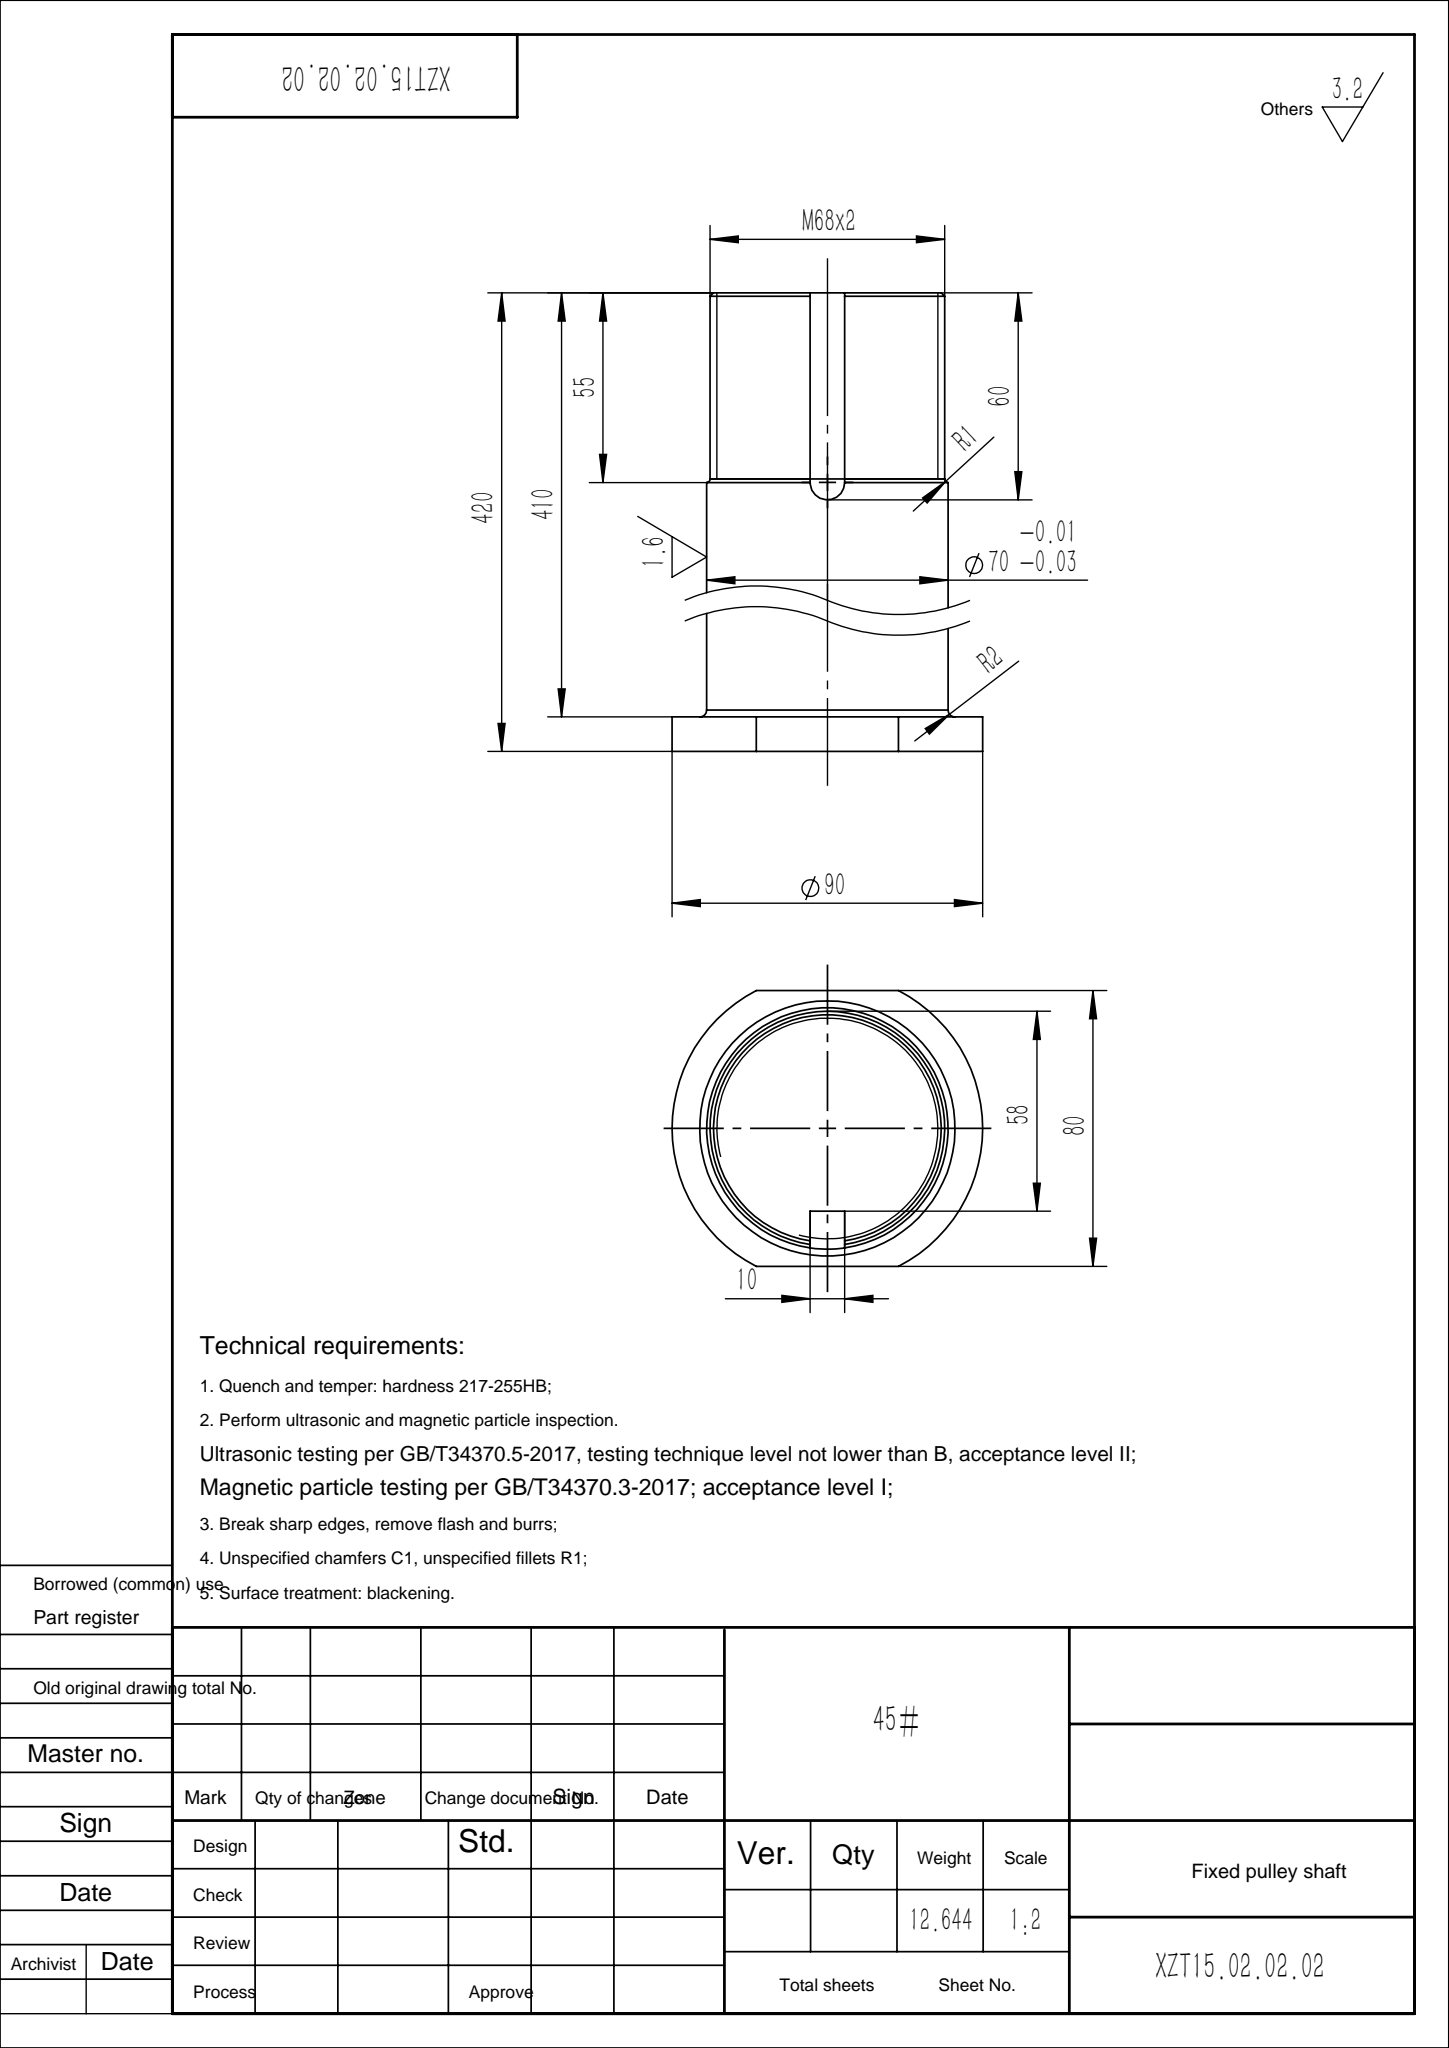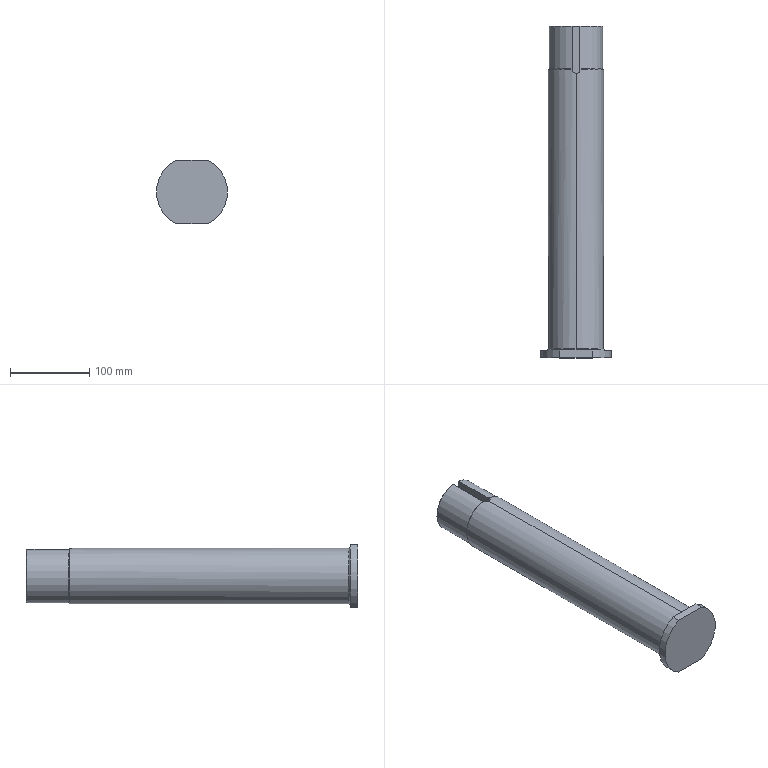Part | SolidWorks | features Fillet 2, ICE 2, Chamfer 1, Revolution 1 | 1 solid | 20 faces | box 90 x 420 x 80 mm | volume 1621053 mm3 | plane 8 | cylinder 6 | torus 4 | cone 2 | commonest cylinder face diameters 70 x2 90 x2 10 x1 68 x1
STEP:
#1=CARTESIAN_POINT('',(0.,10.,37.));
#2=VERTEX_POINT('',#1);
#3=CARTESIAN_POINT('',(0.,10.,-37.));
#4=VERTEX_POINT('',#3);
#5=CARTESIAN_POINT('',(0.,10.,0.));
#6=DIRECTION('',(0.,-1.,0.));
#7=DIRECTION('',(0.,0.,-1.));
#8=AXIS2_PLACEMENT_3D('',#5,#6,#7);
#9=CIRCLE('',#8,37.);
#10=EDGE_CURVE('',#2,#4,#9,.T.);
#11=ORIENTED_EDGE('',*,*,#10,.F.);
#12=CARTESIAN_POINT('',(0.,12.,35.));
#13=VERTEX_POINT('',#12);
#14=CARTESIAN_POINT('',(0.,12.,37.));
#15=DIRECTION('',(1.,0.,0.));
#16=DIRECTION('',(0.,0.,-1.));
#17=AXIS2_PLACEMENT_3D('',#14,#15,#16);
#18=CIRCLE('',#17,2.);
#19=EDGE_CURVE('',#2,#13,#18,.T.);
#20=ORIENTED_EDGE('',*,*,#19,.T.);
#21=CARTESIAN_POINT('',(0.,12.,-35.));
#22=VERTEX_POINT('',#21);
#23=CARTESIAN_POINT('',(0.,12.,0.));
#24=DIRECTION('',(0.,1.,0.));
#25=DIRECTION('',(0.,0.,-1.));
#26=AXIS2_PLACEMENT_3D('',#23,#24,#25);
#27=CIRCLE('',#26,35.);
#28=EDGE_CURVE('',#22,#13,#27,.T.);
#29=ORIENTED_EDGE('',*,*,#28,.F.);
#30=CARTESIAN_POINT('',(0.,12.,-37.));
#31=DIRECTION('',(-1.,0.,0.));
#32=DIRECTION('',(0.,0.,1.));
#33=AXIS2_PLACEMENT_3D('',#30,#31,#32);
#34=CIRCLE('',#33,2.);
#35=EDGE_CURVE('',#4,#22,#34,.T.);
#36=ORIENTED_EDGE('',*,*,#35,.F.);
#37=EDGE_LOOP('',(#11,#20,#29,#36));
#38=FACE_OUTER_BOUND('',#37,.T.);
#39=CARTESIAN_POINT('',(0.,12.,0.));
#40=DIRECTION('',(0.,-1.,0.));
#41=DIRECTION('',(0.,0.,-1.));
#42=AXIS2_PLACEMENT_3D('',#39,#40,#41);
#43=TOROIDAL_SURFACE('',#42,37.,2.);
#44=ADVANCED_FACE('',(#38),#43,.F.);
#45=CARTESIAN_POINT('',(5.,365.,34.641));
#46=VERTEX_POINT('',#45);
#47=CARTESIAN_POINT('',(0.,365.,-35.));
#48=VERTEX_POINT('',#47);
#49=CARTESIAN_POINT('',(0.,365.,0.));
#50=DIRECTION('',(0.,1.,0.));
#51=DIRECTION('',(0.,0.,1.));
#52=AXIS2_PLACEMENT_3D('',#49,#50,#51);
#53=CIRCLE('',#52,35.);
#54=EDGE_CURVE('',#46,#48,#53,.T.);
#55=ORIENTED_EDGE('',*,*,#54,.T.);
#56=CARTESIAN_POINT('',(0.,366.,-34.));
#57=VERTEX_POINT('',#56);
#58=CARTESIAN_POINT('',(0.,366.,-35.));
#59=DIRECTION('',(-1.,0.,0.));
#60=DIRECTION('',(0.,0.,1.));
#61=AXIS2_PLACEMENT_3D('',#58,#59,#60);
#62=CIRCLE('',#61,1.);
#63=EDGE_CURVE('',#48,#57,#62,.T.);
#64=ORIENTED_EDGE('',*,*,#63,.T.);
#65=CARTESIAN_POINT('',(5.,366.,33.63));
#66=VERTEX_POINT('',#65);
#67=CARTESIAN_POINT('',(0.,366.,0.));
#68=DIRECTION('',(0.,1.,0.));
#69=DIRECTION('',(0.,0.,-1.));
#70=AXIS2_PLACEMENT_3D('',#67,#68,#69);
#71=CIRCLE('',#70,34.);
#72=EDGE_CURVE('',#66,#57,#71,.T.);
#73=ORIENTED_EDGE('',*,*,#72,.F.);
#74=CARTESIAN_POINT('',(5.,365.,34.641));
#75=CARTESIAN_POINT('',(5.,365.,34.508));
#76=CARTESIAN_POINT('',(5.,365.026,34.378));
#77=CARTESIAN_POINT('',(5.,365.125,34.134));
#78=CARTESIAN_POINT('',(5.,365.199,34.022));
#79=CARTESIAN_POINT('',(5.,365.475,33.742));
#80=CARTESIAN_POINT('',(5.,365.734,33.63));
#81=CARTESIAN_POINT('',(5.,366.,33.63));
#82=B_SPLINE_CURVE_WITH_KNOTS('',3,(#74,#75,#76,#77,#78,#79,#80,#81),.UNSPECIFIED.,.F.,.F.,(4,2,2,4),(0.,0.0003926,0.0007852,0.00157),.UNSPECIFIED.);
#83=EDGE_CURVE('',#46,#66,#82,.T.);
#84=ORIENTED_EDGE('',*,*,#83,.F.);
#85=EDGE_LOOP('',(#55,#64,#73,#84));
#86=FACE_OUTER_BOUND('',#85,.T.);
#87=CARTESIAN_POINT('',(0.,366.,0.));
#88=DIRECTION('',(0.,-1.,0.));
#89=DIRECTION('',(0.,0.,-1.));
#90=AXIS2_PLACEMENT_3D('',#87,#88,#89);
#91=TOROIDAL_SURFACE('',#90,35.,1.);
#92=ADVANCED_FACE('',(#86),#91,.F.);
#93=CARTESIAN_POINT('',(0.,420.,-33.));
#94=VERTEX_POINT('',#93);
#95=CARTESIAN_POINT('',(-5.,420.,32.619));
#96=VERTEX_POINT('',#95);
#97=CARTESIAN_POINT('',(0.,420.,0.));
#98=DIRECTION('',(0.,1.,0.));
#99=DIRECTION('',(0.,0.,-1.));
#100=AXIS2_PLACEMENT_3D('',#97,#98,#99);
#101=CIRCLE('',#100,33.);
#102=EDGE_CURVE('',#94,#96,#101,.T.);
#103=ORIENTED_EDGE('',*,*,#102,.F.);
#104=CARTESIAN_POINT('',(0.,419.,-34.));
#105=VERTEX_POINT('',#104);
#106=CARTESIAN_POINT('',(0.,420.,-33.));
#107=DIRECTION('',(0.,-0.7071,-0.7071));
#108=VECTOR('',#107,1000.);
#109=LINE('',#106,#108);
#110=EDGE_CURVE('',#94,#105,#109,.T.);
#111=ORIENTED_EDGE('',*,*,#110,.T.);
#112=CARTESIAN_POINT('',(-5.,419.,33.63));
#113=VERTEX_POINT('',#112);
#114=CARTESIAN_POINT('',(0.,419.,0.));
#115=DIRECTION('',(0.,-1.,0.));
#116=DIRECTION('',(0.,0.,-1.));
#117=AXIS2_PLACEMENT_3D('',#114,#115,#116);
#118=CIRCLE('',#117,34.);
#119=EDGE_CURVE('',#113,#105,#118,.T.);
#120=ORIENTED_EDGE('',*,*,#119,.F.);
#121=CARTESIAN_POINT('',(-5.,420.,32.619));
#122=CARTESIAN_POINT('',(-5.,419.667,32.956));
#123=CARTESIAN_POINT('',(-5.,419.333,33.293));
#124=CARTESIAN_POINT('',(-5.,419.,33.63));
#125=B_SPLINE_CURVE_WITH_KNOTS('',3,(#121,#122,#123,#124),.UNSPECIFIED.,.F.,.F.,(4,4),(0.,0.001422),.UNSPECIFIED.);
#126=EDGE_CURVE('',#96,#113,#125,.T.);
#127=ORIENTED_EDGE('',*,*,#126,.F.);
#128=EDGE_LOOP('',(#103,#111,#120,#127));
#129=FACE_OUTER_BOUND('',#128,.T.);
#130=CARTESIAN_POINT('',(0.,420.,0.));
#131=DIRECTION('',(0.,-1.,0.));
#132=DIRECTION('',(0.,0.,-1.));
#133=AXIS2_PLACEMENT_3D('',#130,#131,#132);
#134=CONICAL_SURFACE('',#133,33.,0.7854);
#135=ADVANCED_FACE('',(#129),#134,.T.);
#136=CARTESIAN_POINT('',(0.,12.,0.));
#137=DIRECTION('',(0.,1.,0.));
#138=DIRECTION('',(0.,0.,-1.));
#139=AXIS2_PLACEMENT_3D('',#136,#137,#138);
#140=CIRCLE('',#139,35.);
#141=EDGE_CURVE('',#13,#22,#140,.T.);
#142=ORIENTED_EDGE('',*,*,#141,.T.);
#143=CARTESIAN_POINT('',(0.,0.,-35.));
#144=DIRECTION('',(0.,1.,0.));
#145=VECTOR('',#144,1000.);
#146=LINE('',#143,#145);
#147=EDGE_CURVE('',#22,#48,#146,.T.);
#148=ORIENTED_EDGE('',*,*,#147,.T.);
#149=ORIENTED_EDGE('',*,*,#54,.F.);
#150=CARTESIAN_POINT('',(0.,360.,35.));
#151=VERTEX_POINT('',#150);
#152=CARTESIAN_POINT('',(5.,365.,34.641));
#153=CARTESIAN_POINT('',(5.,364.669,34.641));
#154=CARTESIAN_POINT('',(4.967,364.344,34.646));
#155=CARTESIAN_POINT('',(4.872,363.864,34.659));
#156=CARTESIAN_POINT('',(4.832,363.705,34.665));
#157=CARTESIAN_POINT('',(4.737,363.391,34.678));
#158=CARTESIAN_POINT('',(4.681,363.235,34.686));
#159=CARTESIAN_POINT('',(4.492,362.781,34.711));
#160=CARTESIAN_POINT('',(4.339,362.494,34.731));
#161=CARTESIAN_POINT('',(3.976,361.95,34.774));
#162=CARTESIAN_POINT('',(3.765,361.693,34.798));
#163=CARTESIAN_POINT('',(3.304,361.233,34.845));
#164=CARTESIAN_POINT('',(3.052,361.026,34.868));
#165=CARTESIAN_POINT('',(2.505,360.66,34.911));
#166=CARTESIAN_POINT('',(2.215,360.505,34.931));
#167=CARTESIAN_POINT('',(1.613,360.256,34.964));
#168=CARTESIAN_POINT('',(1.297,360.16,34.977));
#169=CARTESIAN_POINT('',(0.6515,360.032,34.995));
#170=CARTESIAN_POINT('',(0.3267,360.,35.));
#171=CARTESIAN_POINT('',(0.,360.,35.));
#172=B_SPLINE_CURVE_WITH_KNOTS('',3,(#152,#153,#154,#155,#156,#157,#158,#159,#160,#161,#162,#163,#164,#165,#166,#167,#168,#169,#170,#171),.UNSPECIFIED.,.F.,.F.,(4,2,2,2,2,2,2,2,2,4),(0.,0.0009785,0.001468,0.001957,0.002935,0.003914,0.004892,0.005871,0.006849,0.007828),.UNSPECIFIED.);
#173=EDGE_CURVE('',#46,#151,#172,.T.);
#174=ORIENTED_EDGE('',*,*,#173,.T.);
#175=CARTESIAN_POINT('',(0.,0.,35.));
#176=DIRECTION('',(0.,1.,0.));
#177=VECTOR('',#176,1000.);
#178=LINE('',#175,#177);
#179=EDGE_CURVE('',#13,#151,#178,.T.);
#180=ORIENTED_EDGE('',*,*,#179,.F.);
#181=EDGE_LOOP('',(#142,#148,#149,#174,#180));
#182=FACE_OUTER_BOUND('',#181,.T.);
#183=CARTESIAN_POINT('',(0.,0.,0.));
#184=DIRECTION('',(0.,1.,0.));
#185=DIRECTION('',(0.,0.,1.));
#186=AXIS2_PLACEMENT_3D('',#183,#184,#185);
#187=CYLINDRICAL_SURFACE('',#186,35.);
#188=ADVANCED_FACE('',(#182),#187,.T.);
#189=ORIENTED_EDGE('',*,*,#147,.F.);
#190=ORIENTED_EDGE('',*,*,#28,.T.);
#191=ORIENTED_EDGE('',*,*,#179,.T.);
#192=CARTESIAN_POINT('',(-5.,365.,34.641));
#193=VERTEX_POINT('',#192);
#194=CARTESIAN_POINT('',(0.,360.,35.));
#195=CARTESIAN_POINT('',(-0.3264,360.,35.));
#196=CARTESIAN_POINT('',(-0.6579,360.033,34.995));
#197=CARTESIAN_POINT('',(-1.299,360.161,34.977));
#198=CARTESIAN_POINT('',(-1.611,360.255,34.964));
#199=CARTESIAN_POINT('',(-2.065,360.443,34.939));
#200=CARTESIAN_POINT('',(-2.215,360.514,34.93));
#201=CARTESIAN_POINT('',(-2.504,360.669,34.911));
#202=CARTESIAN_POINT('',(-2.643,360.753,34.9));
#203=CARTESIAN_POINT('',(-3.049,361.024,34.868));
#204=CARTESIAN_POINT('',(-3.302,361.231,34.845));
#205=CARTESIAN_POINT('',(-3.768,361.696,34.797));
#206=CARTESIAN_POINT('',(-3.974,361.948,34.774));
#207=CARTESIAN_POINT('',(-4.336,362.489,34.731));
#208=CARTESIAN_POINT('',(-4.493,362.781,34.711));
#209=CARTESIAN_POINT('',(-4.744,363.386,34.677));
#210=CARTESIAN_POINT('',(-4.838,363.697,34.664));
#211=CARTESIAN_POINT('',(-4.967,364.338,34.646));
#212=CARTESIAN_POINT('',(-5.,364.669,34.641));
#213=CARTESIAN_POINT('',(-5.,365.,34.641));
#214=B_SPLINE_CURVE_WITH_KNOTS('',3,(#194,#195,#196,#197,#198,#199,#200,#201,#202,#203,#204,#205,#206,#207,#208,#209,#210,#211,#212,#213),.UNSPECIFIED.,.F.,.F.,(4,2,2,2,2,2,2,2,2,4),(0.007828,0.008806,0.009783,0.01027,0.01076,0.01174,0.01272,0.01369,0.01467,0.01565),.UNSPECIFIED.);
#215=EDGE_CURVE('',#151,#193,#214,.T.);
#216=ORIENTED_EDGE('',*,*,#215,.T.);
#217=CARTESIAN_POINT('',(0.,365.,0.));
#218=DIRECTION('',(0.,1.,0.));
#219=DIRECTION('',(0.,0.,1.));
#220=AXIS2_PLACEMENT_3D('',#217,#218,#219);
#221=CIRCLE('',#220,35.);
#222=EDGE_CURVE('',#48,#193,#221,.T.);
#223=ORIENTED_EDGE('',*,*,#222,.F.);
#224=EDGE_LOOP('',(#189,#190,#191,#216,#223));
#225=FACE_OUTER_BOUND('',#224,.T.);
#226=CARTESIAN_POINT('',(0.,0.,0.));
#227=DIRECTION('',(0.,1.,0.));
#228=DIRECTION('',(0.,0.,1.));
#229=AXIS2_PLACEMENT_3D('',#226,#227,#228);
#230=CYLINDRICAL_SURFACE('',#229,35.);
#231=ADVANCED_FACE('',(#225),#230,.T.);
#232=CARTESIAN_POINT('',(5.,419.,33.63));
#233=VERTEX_POINT('',#232);
#234=CARTESIAN_POINT('',(5.,0.,33.63));
#235=DIRECTION('',(0.,-1.,0.));
#236=VECTOR('',#235,1000.);
#237=LINE('',#234,#236);
#238=EDGE_CURVE('',#233,#66,#237,.T.);
#239=ORIENTED_EDGE('',*,*,#238,.T.);
#240=ORIENTED_EDGE('',*,*,#72,.T.);
#241=CARTESIAN_POINT('',(-5.,366.,33.63));
#242=VERTEX_POINT('',#241);
#243=CARTESIAN_POINT('',(0.,366.,0.));
#244=DIRECTION('',(0.,1.,0.));
#245=DIRECTION('',(0.,0.,-1.));
#246=AXIS2_PLACEMENT_3D('',#243,#244,#245);
#247=CIRCLE('',#246,34.);
#248=EDGE_CURVE('',#57,#242,#247,.T.);
#249=ORIENTED_EDGE('',*,*,#248,.T.);
#250=CARTESIAN_POINT('',(-5.,0.,33.63));
#251=DIRECTION('',(0.,1.,0.));
#252=VECTOR('',#251,1000.);
#253=LINE('',#250,#252);
#254=EDGE_CURVE('',#242,#113,#253,.T.);
#255=ORIENTED_EDGE('',*,*,#254,.T.);
#256=ORIENTED_EDGE('',*,*,#119,.T.);
#257=CARTESIAN_POINT('',(0.,419.,0.));
#258=DIRECTION('',(0.,-1.,0.));
#259=DIRECTION('',(0.,0.,-1.));
#260=AXIS2_PLACEMENT_3D('',#257,#258,#259);
#261=CIRCLE('',#260,34.);
#262=EDGE_CURVE('',#105,#233,#261,.T.);
#263=ORIENTED_EDGE('',*,*,#262,.T.);
#264=EDGE_LOOP('',(#239,#240,#249,#255,#256,#263));
#265=FACE_OUTER_BOUND('',#264,.T.);
#266=CARTESIAN_POINT('',(0.,0.,0.));
#267=DIRECTION('',(0.,1.,0.));
#268=DIRECTION('',(0.,0.,1.));
#269=AXIS2_PLACEMENT_3D('',#266,#267,#268);
#270=CYLINDRICAL_SURFACE('',#269,34.);
#271=ADVANCED_FACE('',(#265),#270,.T.);
#272=CARTESIAN_POINT('',(5.,420.,24.));
#273=VERTEX_POINT('',#272);
#274=CARTESIAN_POINT('',(5.,420.,32.619));
#275=VERTEX_POINT('',#274);
#276=CARTESIAN_POINT('',(5.,420.,40.001));
#277=DIRECTION('',(0.,0.,1.));
#278=VECTOR('',#277,1000.);
#279=LINE('',#276,#278);
#280=EDGE_CURVE('',#273,#275,#279,.T.);
#281=ORIENTED_EDGE('',*,*,#280,.T.);
#282=CARTESIAN_POINT('',(0.,420.,0.));
#283=DIRECTION('',(0.,1.,0.));
#284=DIRECTION('',(0.,0.,-1.));
#285=AXIS2_PLACEMENT_3D('',#282,#283,#284);
#286=CIRCLE('',#285,33.);
#287=EDGE_CURVE('',#275,#94,#286,.T.);
#288=ORIENTED_EDGE('',*,*,#287,.T.);
#289=ORIENTED_EDGE('',*,*,#102,.T.);
#290=CARTESIAN_POINT('',(-5.,420.,24.));
#291=VERTEX_POINT('',#290);
#292=CARTESIAN_POINT('',(-5.,420.,40.001));
#293=DIRECTION('',(0.,0.,-1.));
#294=VECTOR('',#293,1000.);
#295=LINE('',#292,#294);
#296=EDGE_CURVE('',#96,#291,#295,.T.);
#297=ORIENTED_EDGE('',*,*,#296,.T.);
#298=CARTESIAN_POINT('',(0.,420.,24.));
#299=DIRECTION('',(1.,0.,0.));
#300=VECTOR('',#299,1000.);
#301=LINE('',#298,#300);
#302=EDGE_CURVE('',#291,#273,#301,.T.);
#303=ORIENTED_EDGE('',*,*,#302,.T.);
#304=EDGE_LOOP('',(#281,#288,#289,#297,#303));
#305=FACE_OUTER_BOUND('',#304,.T.);
#306=CARTESIAN_POINT('',(34.,420.,0.));
#307=DIRECTION('',(0.,-1.,0.));
#308=DIRECTION('',(0.,0.,-1.));
#309=AXIS2_PLACEMENT_3D('',#306,#307,#308);
#310=PLANE('',#309);
#311=ADVANCED_FACE('',(#305),#310,.F.);
#312=CARTESIAN_POINT('',(-20.616,0.,-40.));
#313=VERTEX_POINT('',#312);
#314=CARTESIAN_POINT('',(-20.616,0.,40.));
#315=VERTEX_POINT('',#314);
#316=CARTESIAN_POINT('',(0.,0.,0.));
#317=DIRECTION('',(0.,1.,0.));
#318=DIRECTION('',(0.,0.,1.));
#319=AXIS2_PLACEMENT_3D('',#316,#317,#318);
#320=CIRCLE('',#319,45.);
#321=EDGE_CURVE('',#313,#315,#320,.T.);
#322=ORIENTED_EDGE('',*,*,#321,.T.);
#323=CARTESIAN_POINT('',(-20.616,10.,40.));
#324=VERTEX_POINT('',#323);
#325=CARTESIAN_POINT('',(-20.616,0.,40.));
#326=DIRECTION('',(0.,1.,0.));
#327=VECTOR('',#326,1000.);
#328=LINE('',#325,#327);
#329=EDGE_CURVE('',#315,#324,#328,.T.);
#330=ORIENTED_EDGE('',*,*,#329,.T.);
#331=CARTESIAN_POINT('',(-20.616,10.,-40.));
#332=VERTEX_POINT('',#331);
#333=CARTESIAN_POINT('',(0.,10.,0.));
#334=DIRECTION('',(0.,1.,0.));
#335=DIRECTION('',(0.,0.,1.));
#336=AXIS2_PLACEMENT_3D('',#333,#334,#335);
#337=CIRCLE('',#336,45.);
#338=EDGE_CURVE('',#332,#324,#337,.T.);
#339=ORIENTED_EDGE('',*,*,#338,.F.);
#340=CARTESIAN_POINT('',(-20.616,0.,-40.));
#341=DIRECTION('',(0.,-1.,0.));
#342=VECTOR('',#341,1000.);
#343=LINE('',#340,#342);
#344=EDGE_CURVE('',#332,#313,#343,.T.);
#345=ORIENTED_EDGE('',*,*,#344,.T.);
#346=EDGE_LOOP('',(#322,#330,#339,#345));
#347=FACE_OUTER_BOUND('',#346,.T.);
#348=CARTESIAN_POINT('',(0.,0.,0.));
#349=DIRECTION('',(0.,1.,0.));
#350=DIRECTION('',(0.,0.,1.));
#351=AXIS2_PLACEMENT_3D('',#348,#349,#350);
#352=CYLINDRICAL_SURFACE('',#351,45.);
#353=ADVANCED_FACE('',(#347),#352,.T.);
#354=CARTESIAN_POINT('',(20.616,0.,40.));
#355=VERTEX_POINT('',#354);
#356=CARTESIAN_POINT('',(20.616,0.,-40.));
#357=VERTEX_POINT('',#356);
#358=CARTESIAN_POINT('',(0.,0.,0.));
#359=DIRECTION('',(0.,1.,0.));
#360=DIRECTION('',(0.,0.,1.));
#361=AXIS2_PLACEMENT_3D('',#358,#359,#360);
#362=CIRCLE('',#361,45.);
#363=EDGE_CURVE('',#355,#357,#362,.T.);
#364=ORIENTED_EDGE('',*,*,#363,.F.);
#365=CARTESIAN_POINT('',(65.,0.,40.));
#366=DIRECTION('',(1.,0.,0.));
#367=VECTOR('',#366,1000.);
#368=LINE('',#365,#367);
#369=EDGE_CURVE('',#315,#355,#368,.T.);
#370=ORIENTED_EDGE('',*,*,#369,.F.);
#371=ORIENTED_EDGE('',*,*,#321,.F.);
#372=CARTESIAN_POINT('',(65.,0.,-40.));
#373=DIRECTION('',(-1.,0.,0.));
#374=VECTOR('',#373,1000.);
#375=LINE('',#372,#374);
#376=EDGE_CURVE('',#357,#313,#375,.T.);
#377=ORIENTED_EDGE('',*,*,#376,.F.);
#378=EDGE_LOOP('',(#364,#370,#371,#377));
#379=FACE_OUTER_BOUND('',#378,.T.);
#380=CARTESIAN_POINT('',(0.,0.,0.));
#381=DIRECTION('',(0.,1.,0.));
#382=DIRECTION('',(0.,0.,1.));
#383=AXIS2_PLACEMENT_3D('',#380,#381,#382);
#384=PLANE('',#383);
#385=ADVANCED_FACE('',(#379),#384,.F.);
#386=CARTESIAN_POINT('',(20.616,10.,40.));
#387=VERTEX_POINT('',#386);
#388=CARTESIAN_POINT('',(20.616,10.,-40.));
#389=VERTEX_POINT('',#388);
#390=CARTESIAN_POINT('',(0.,10.,0.));
#391=DIRECTION('',(0.,1.,0.));
#392=DIRECTION('',(0.,0.,1.));
#393=AXIS2_PLACEMENT_3D('',#390,#391,#392);
#394=CIRCLE('',#393,45.);
#395=EDGE_CURVE('',#387,#389,#394,.T.);
#396=ORIENTED_EDGE('',*,*,#395,.F.);
#397=CARTESIAN_POINT('',(20.616,0.,40.));
#398=DIRECTION('',(0.,-1.,0.));
#399=VECTOR('',#398,1000.);
#400=LINE('',#397,#399);
#401=EDGE_CURVE('',#387,#355,#400,.T.);
#402=ORIENTED_EDGE('',*,*,#401,.T.);
#403=ORIENTED_EDGE('',*,*,#363,.T.);
#404=CARTESIAN_POINT('',(20.616,0.,-40.));
#405=DIRECTION('',(0.,1.,0.));
#406=VECTOR('',#405,1000.);
#407=LINE('',#404,#406);
#408=EDGE_CURVE('',#357,#389,#407,.T.);
#409=ORIENTED_EDGE('',*,*,#408,.T.);
#410=EDGE_LOOP('',(#396,#402,#403,#409));
#411=FACE_OUTER_BOUND('',#410,.T.);
#412=CARTESIAN_POINT('',(0.,0.,0.));
#413=DIRECTION('',(0.,1.,0.));
#414=DIRECTION('',(0.,0.,1.));
#415=AXIS2_PLACEMENT_3D('',#412,#413,#414);
#416=CYLINDRICAL_SURFACE('',#415,45.);
#417=ADVANCED_FACE('',(#411),#416,.T.);
#418=CARTESIAN_POINT('',(0.,10.,0.));
#419=DIRECTION('',(0.,-1.,0.));
#420=DIRECTION('',(0.,0.,-1.));
#421=AXIS2_PLACEMENT_3D('',#418,#419,#420);
#422=CIRCLE('',#421,37.);
#423=EDGE_CURVE('',#4,#2,#422,.T.);
#424=ORIENTED_EDGE('',*,*,#423,.T.);
#425=ORIENTED_EDGE('',*,*,#10,.T.);
#426=EDGE_LOOP('',(#424,#425));
#427=FACE_BOUND('',#426,.T.);
#428=ORIENTED_EDGE('',*,*,#338,.T.);
#429=CARTESIAN_POINT('',(45.,10.,40.));
#430=DIRECTION('',(1.,0.,0.));
#431=VECTOR('',#430,1000.);
#432=LINE('',#429,#431);
#433=EDGE_CURVE('',#324,#387,#432,.T.);
#434=ORIENTED_EDGE('',*,*,#433,.T.);
#435=ORIENTED_EDGE('',*,*,#395,.T.);
#436=CARTESIAN_POINT('',(45.,10.,-40.));
#437=DIRECTION('',(-1.,0.,0.));
#438=VECTOR('',#437,1000.);
#439=LINE('',#436,#438);
#440=EDGE_CURVE('',#389,#332,#439,.T.);
#441=ORIENTED_EDGE('',*,*,#440,.T.);
#442=EDGE_LOOP('',(#428,#434,#435,#441));
#443=FACE_OUTER_BOUND('',#442,.T.);
#444=CARTESIAN_POINT('',(45.,10.,0.));
#445=DIRECTION('',(0.,-1.,0.));
#446=DIRECTION('',(0.,0.,-1.));
#447=AXIS2_PLACEMENT_3D('',#444,#445,#446);
#448=PLANE('',#447);
#449=ADVANCED_FACE('',(#427,#443),#448,.F.);
#450=ORIENTED_EDGE('',*,*,#376,.T.);
#451=ORIENTED_EDGE('',*,*,#344,.F.);
#452=ORIENTED_EDGE('',*,*,#440,.F.);
#453=ORIENTED_EDGE('',*,*,#408,.F.);
#454=EDGE_LOOP('',(#450,#451,#452,#453));
#455=FACE_OUTER_BOUND('',#454,.T.);
#456=CARTESIAN_POINT('',(65.,10.,-40.));
#457=DIRECTION('',(0.,0.,1.));
#458=DIRECTION('',(1.,0.,0.));
#459=AXIS2_PLACEMENT_3D('',#456,#457,#458);
#460=PLANE('',#459);
#461=ADVANCED_FACE('',(#455),#460,.F.);
#462=ORIENTED_EDGE('',*,*,#369,.T.);
#463=ORIENTED_EDGE('',*,*,#401,.F.);
#464=ORIENTED_EDGE('',*,*,#433,.F.);
#465=ORIENTED_EDGE('',*,*,#329,.F.);
#466=EDGE_LOOP('',(#462,#463,#464,#465));
#467=FACE_OUTER_BOUND('',#466,.T.);
#468=CARTESIAN_POINT('',(65.,10.,40.));
#469=DIRECTION('',(0.,0.,-1.));
#470=DIRECTION('',(-1.,0.,0.));
#471=AXIS2_PLACEMENT_3D('',#468,#469,#470);
#472=PLANE('',#471);
#473=ADVANCED_FACE('',(#467),#472,.F.);
#474=ORIENTED_EDGE('',*,*,#296,.F.);
#475=ORIENTED_EDGE('',*,*,#126,.T.);
#476=ORIENTED_EDGE('',*,*,#254,.F.);
#477=CARTESIAN_POINT('',(-5.,366.,33.63));
#478=CARTESIAN_POINT('',(-5.,365.867,33.63));
#479=CARTESIAN_POINT('',(-5.,365.737,33.657));
#480=CARTESIAN_POINT('',(-5.,365.494,33.759));
#481=CARTESIAN_POINT('',(-5.,365.383,33.835));
#482=CARTESIAN_POINT('',(-5.,365.199,34.021));
#483=CARTESIAN_POINT('',(-5.,365.125,34.134));
#484=CARTESIAN_POINT('',(-5.,365.026,34.376));
#485=CARTESIAN_POINT('',(-5.,365.,34.508));
#486=CARTESIAN_POINT('',(-5.,365.,34.641));
#487=B_SPLINE_CURVE_WITH_KNOTS('',3,(#477,#478,#479,#480,#481,#482,#483,#484,#485,#486),.UNSPECIFIED.,.F.,.F.,(4,2,2,2,4),(0.,0.0003926,0.0007852,0.001178,0.00157),.UNSPECIFIED.);
#488=EDGE_CURVE('',#242,#193,#487,.T.);
#489=ORIENTED_EDGE('',*,*,#488,.T.);
#490=CARTESIAN_POINT('',(-5.,365.,24.));
#491=VERTEX_POINT('',#490);
#492=CARTESIAN_POINT('',(-5.,365.,40.001));
#493=DIRECTION('',(0.,0.,-1.));
#494=VECTOR('',#493,1000.);
#495=LINE('',#492,#494);
#496=EDGE_CURVE('',#193,#491,#495,.T.);
#497=ORIENTED_EDGE('',*,*,#496,.T.);
#498=CARTESIAN_POINT('',(-5.,420.,24.));
#499=DIRECTION('',(0.,-1.,0.));
#500=VECTOR('',#499,1000.);
#501=LINE('',#498,#500);
#502=EDGE_CURVE('',#291,#491,#501,.T.);
#503=ORIENTED_EDGE('',*,*,#502,.F.);
#504=EDGE_LOOP('',(#474,#475,#476,#489,#497,#503));
#505=FACE_OUTER_BOUND('',#504,.T.);
#506=CARTESIAN_POINT('',(-5.,420.,40.001));
#507=DIRECTION('',(1.,0.,0.));
#508=DIRECTION('',(0.,1.,0.));
#509=AXIS2_PLACEMENT_3D('',#506,#507,#508);
#510=PLANE('',#509);
#511=ADVANCED_FACE('',(#505),#510,.T.);
#512=ORIENTED_EDGE('',*,*,#173,.F.);
#513=CARTESIAN_POINT('',(5.,365.,24.));
#514=VERTEX_POINT('',#513);
#515=CARTESIAN_POINT('',(5.,365.,40.001));
#516=DIRECTION('',(0.,0.,-1.));
#517=VECTOR('',#516,1000.);
#518=LINE('',#515,#517);
#519=EDGE_CURVE('',#46,#514,#518,.T.);
#520=ORIENTED_EDGE('',*,*,#519,.T.);
#521=CARTESIAN_POINT('',(0.,365.,24.));
#522=DIRECTION('',(0.,0.,1.));
#523=DIRECTION('',(1.,0.,0.));
#524=AXIS2_PLACEMENT_3D('',#521,#522,#523);
#525=CIRCLE('',#524,5.);
#526=EDGE_CURVE('',#491,#514,#525,.T.);
#527=ORIENTED_EDGE('',*,*,#526,.F.);
#528=ORIENTED_EDGE('',*,*,#496,.F.);
#529=ORIENTED_EDGE('',*,*,#215,.F.);
#530=EDGE_LOOP('',(#512,#520,#527,#528,#529));
#531=FACE_OUTER_BOUND('',#530,.T.);
#532=CARTESIAN_POINT('',(0.,365.,40.001));
#533=DIRECTION('',(0.,0.,-1.));
#534=DIRECTION('',(-1.,0.,0.));
#535=AXIS2_PLACEMENT_3D('',#532,#533,#534);
#536=CYLINDRICAL_SURFACE('',#535,5.);
#537=ADVANCED_FACE('',(#531),#536,.F.);
#538=ORIENTED_EDGE('',*,*,#238,.F.);
#539=CARTESIAN_POINT('',(5.,419.,33.63));
#540=CARTESIAN_POINT('',(5.,419.333,33.293));
#541=CARTESIAN_POINT('',(5.,419.667,32.956));
#542=CARTESIAN_POINT('',(5.,420.,32.619));
#543=B_SPLINE_CURVE_WITH_KNOTS('',3,(#539,#540,#541,#542),.UNSPECIFIED.,.F.,.F.,(4,4),(0.,0.001422),.UNSPECIFIED.);
#544=EDGE_CURVE('',#233,#275,#543,.T.);
#545=ORIENTED_EDGE('',*,*,#544,.T.);
#546=ORIENTED_EDGE('',*,*,#280,.F.);
#547=CARTESIAN_POINT('',(5.,420.,24.));
#548=DIRECTION('',(0.,1.,0.));
#549=VECTOR('',#548,1000.);
#550=LINE('',#547,#549);
#551=EDGE_CURVE('',#514,#273,#550,.T.);
#552=ORIENTED_EDGE('',*,*,#551,.F.);
#553=ORIENTED_EDGE('',*,*,#519,.F.);
#554=ORIENTED_EDGE('',*,*,#83,.T.);
#555=EDGE_LOOP('',(#538,#545,#546,#552,#553,#554));
#556=FACE_OUTER_BOUND('',#555,.T.);
#557=CARTESIAN_POINT('',(5.,420.,40.001));
#558=DIRECTION('',(-1.,0.,0.));
#559=DIRECTION('',(0.,-1.,0.));
#560=AXIS2_PLACEMENT_3D('',#557,#558,#559);
#561=PLANE('',#560);
#562=ADVANCED_FACE('',(#556),#561,.T.);
#563=ORIENTED_EDGE('',*,*,#502,.T.);
#564=ORIENTED_EDGE('',*,*,#526,.T.);
#565=ORIENTED_EDGE('',*,*,#551,.T.);
#566=ORIENTED_EDGE('',*,*,#302,.F.);
#567=EDGE_LOOP('',(#563,#564,#565,#566));
#568=FACE_OUTER_BOUND('',#567,.T.);
#569=CARTESIAN_POINT('',(0.,420.,24.));
#570=DIRECTION('',(0.,0.,1.));
#571=DIRECTION('',(1.,0.,0.));
#572=AXIS2_PLACEMENT_3D('',#569,#570,#571);
#573=PLANE('',#572);
#574=ADVANCED_FACE('',(#568),#573,.T.);
#575=ORIENTED_EDGE('',*,*,#110,.F.);
#576=ORIENTED_EDGE('',*,*,#287,.F.);
#577=ORIENTED_EDGE('',*,*,#544,.F.);
#578=ORIENTED_EDGE('',*,*,#262,.F.);
#579=EDGE_LOOP('',(#575,#576,#577,#578));
#580=FACE_OUTER_BOUND('',#579,.T.);
#581=CARTESIAN_POINT('',(0.,420.,0.));
#582=DIRECTION('',(0.,-1.,0.));
#583=DIRECTION('',(0.,0.,-1.));
#584=AXIS2_PLACEMENT_3D('',#581,#582,#583);
#585=CONICAL_SURFACE('',#584,33.,0.7854);
#586=ADVANCED_FACE('',(#580),#585,.T.);
#587=ORIENTED_EDGE('',*,*,#63,.F.);
#588=ORIENTED_EDGE('',*,*,#222,.T.);
#589=ORIENTED_EDGE('',*,*,#488,.F.);
#590=ORIENTED_EDGE('',*,*,#248,.F.);
#591=EDGE_LOOP('',(#587,#588,#589,#590));
#592=FACE_OUTER_BOUND('',#591,.T.);
#593=CARTESIAN_POINT('',(0.,366.,0.));
#594=DIRECTION('',(0.,-1.,0.));
#595=DIRECTION('',(0.,0.,-1.));
#596=AXIS2_PLACEMENT_3D('',#593,#594,#595);
#597=TOROIDAL_SURFACE('',#596,35.,1.);
#598=ADVANCED_FACE('',(#592),#597,.F.);
#599=ORIENTED_EDGE('',*,*,#19,.F.);
#600=ORIENTED_EDGE('',*,*,#423,.F.);
#601=ORIENTED_EDGE('',*,*,#35,.T.);
#602=ORIENTED_EDGE('',*,*,#141,.F.);
#603=EDGE_LOOP('',(#599,#600,#601,#602));
#604=FACE_OUTER_BOUND('',#603,.T.);
#605=CARTESIAN_POINT('',(0.,12.,0.));
#606=DIRECTION('',(0.,-1.,0.));
#607=DIRECTION('',(0.,0.,-1.));
#608=AXIS2_PLACEMENT_3D('',#605,#606,#607);
#609=TOROIDAL_SURFACE('',#608,37.,2.);
#610=ADVANCED_FACE('',(#604),#609,.F.);
#611=CLOSED_SHELL('',(#44,#92,#135,#188,#231,#271,#311,#353,#385,#417,#449,#461,#473,#511,#537,#562,#574,#586,#598,#610));
#612=MANIFOLD_SOLID_BREP('',#611);
#613=CARTESIAN_POINT('',(0.,0.,0.));
#614=DIRECTION('',(0.,0.,1.));
#615=DIRECTION('',(1.,0.,0.));
#616=AXIS2_PLACEMENT_3D('',#613,#614,#615);
#617=(LENGTH_UNIT()NAMED_UNIT(*)SI_UNIT(.MILLI.,.METRE.));
#618=UNCERTAINTY_MEASURE_WITH_UNIT(LENGTH_MEASURE(0.00001),#617,'','');
#619=(NAMED_UNIT(*)PLANE_ANGLE_UNIT()SI_UNIT($,.RADIAN.));
#620=(NAMED_UNIT(*)SI_UNIT($,.STERADIAN.)SOLID_ANGLE_UNIT());
#621=(GEOMETRIC_REPRESENTATION_CONTEXT(3)GLOBAL_UNCERTAINTY_ASSIGNED_CONTEXT((#618))GLOBAL_UNIT_ASSIGNED_CONTEXT((#617,#619,#620))REPRESENTATION_CONTEXT('',''));
#622=ADVANCED_BREP_SHAPE_REPRESENTATION('',(#612,#616),#621);